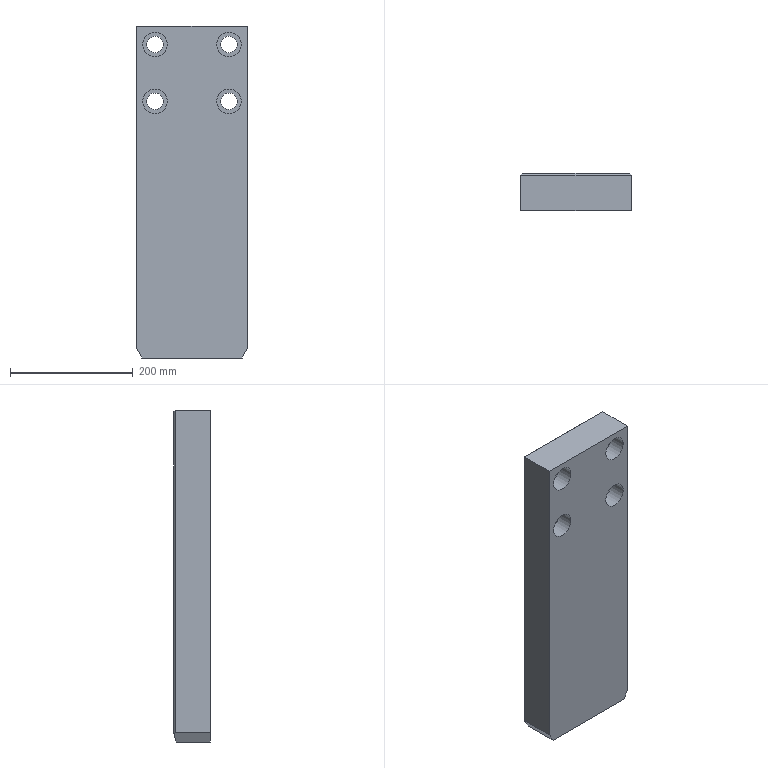Part | NX | features FD 2 | 1 solid | 26 faces | box 180 x 60 x 540 mm | volume 5599611 mm3 | plane 16 | cylinder 9 | cone 1 | commonest cylinder face diameters 27 x4 40 x4 10.2 x1
STEP:
#1=CARTESIAN_POINT('',(2475.,-645.5,147.5));
#2=VERTEX_POINT('',#1);
#3=CARTESIAN_POINT('',(2475.,-645.5,134.));
#4=DIRECTION('',(0.,-1.,0.));
#5=DIRECTION('',(0.,0.,1.));
#6=AXIS2_PLACEMENT_3D('',#3,#4,#5);
#7=CIRCLE('',#6,13.5);
#8=EDGE_CURVE('',#2,#2,#7,.T.);
#9=ORIENTED_EDGE('',*,*,#8,.F.);
#10=EDGE_LOOP('',(#9));
#11=FACE_BOUND('',#10,.T.);
#12=CARTESIAN_POINT('',(2475.,-645.5,154.));
#13=VERTEX_POINT('',#12);
#14=CARTESIAN_POINT('',(2475.,-645.5,134.));
#15=DIRECTION('',(0.,1.,0.));
#16=DIRECTION('',(0.,0.,1.));
#17=AXIS2_PLACEMENT_3D('',#14,#15,#16);
#18=CIRCLE('',#17,20.);
#19=EDGE_CURVE('',#13,#13,#18,.T.);
#20=ORIENTED_EDGE('',*,*,#19,.F.);
#21=EDGE_LOOP('',(#20));
#22=FACE_BOUND('',#21,.T.);
#23=CARTESIAN_POINT('',(2475.,-645.5,134.));
#24=DIRECTION('',(0.,1.,0.));
#25=DIRECTION('',(0.,0.,-1.));
#26=AXIS2_PLACEMENT_3D('',#23,#24,#25);
#27=PLANE('',#26);
#28=ADVANCED_FACE('',(#11,#22),#27,.F.);
#29=CARTESIAN_POINT('',(2475.,-672.5,154.));
#30=VERTEX_POINT('',#29);
#31=CARTESIAN_POINT('',(2475.,-672.5,134.));
#32=DIRECTION('',(0.,1.,0.));
#33=DIRECTION('',(0.,0.,1.));
#34=AXIS2_PLACEMENT_3D('',#31,#32,#33);
#35=CIRCLE('',#34,20.);
#36=EDGE_CURVE('',#30,#30,#35,.T.);
#37=ORIENTED_EDGE('',*,*,#36,.F.);
#38=EDGE_LOOP('',(#37));
#39=FACE_BOUND('',#38,.T.);
#40=ORIENTED_EDGE('',*,*,#19,.T.);
#41=EDGE_LOOP('',(#40));
#42=FACE_BOUND('',#41,.T.);
#43=CARTESIAN_POINT('',(2475.,-656.5,134.));
#44=DIRECTION('',(0.,1.,0.));
#45=DIRECTION('',(0.,0.,-1.));
#46=AXIS2_PLACEMENT_3D('',#43,#44,#45);
#47=CYLINDRICAL_SURFACE('',#46,20.);
#48=ADVANCED_FACE('',(#39,#42),#47,.F.);
#49=ORIENTED_EDGE('',*,*,#8,.T.);
#50=EDGE_LOOP('',(#49));
#51=FACE_BOUND('',#50,.T.);
#52=CARTESIAN_POINT('',(2475.,-612.5,147.5));
#53=VERTEX_POINT('',#52);
#54=CARTESIAN_POINT('',(2475.,-612.5,134.));
#55=DIRECTION('',(0.,1.,0.));
#56=DIRECTION('',(0.,0.,1.));
#57=AXIS2_PLACEMENT_3D('',#54,#55,#56);
#58=CIRCLE('',#57,13.5);
#59=EDGE_CURVE('',#53,#53,#58,.T.);
#60=ORIENTED_EDGE('',*,*,#59,.T.);
#61=EDGE_LOOP('',(#60));
#62=FACE_BOUND('',#61,.T.);
#63=CARTESIAN_POINT('',(2475.,-640.,134.));
#64=DIRECTION('',(0.,1.,0.));
#65=DIRECTION('',(0.,0.,-1.));
#66=AXIS2_PLACEMENT_3D('',#63,#64,#65);
#67=CYLINDRICAL_SURFACE('',#66,13.5);
#68=ADVANCED_FACE('',(#51,#62),#67,.F.);
#69=CARTESIAN_POINT('',(2415.,-637.4,-251.5));
#70=VERTEX_POINT('',#69);
#71=CARTESIAN_POINT('',(2415.,-642.5,-251.5));
#72=DIRECTION('',(0.,0.,1.));
#73=DIRECTION('',(0.,1.,0.));
#74=AXIS2_PLACEMENT_3D('',#71,#72,#73);
#75=CIRCLE('',#74,5.1);
#76=EDGE_CURVE('',#70,#70,#75,.T.);
#77=ORIENTED_EDGE('',*,*,#76,.F.);
#78=EDGE_LOOP('',(#77));
#79=FACE_BOUND('',#78,.T.);
#80=CARTESIAN_POINT('',(2415.,-642.5,-248.556));
#81=VERTEX_POINT('',#80);
#82=VERTEX_LOOP('',#81);
#83=FACE_BOUND('',#82,.T.);
#84=CARTESIAN_POINT('',(2415.,-642.5,-250.028));
#85=DIRECTION('',(0.,0.,-1.));
#86=DIRECTION('',(0.,1.,0.));
#87=AXIS2_PLACEMENT_3D('',#84,#85,#86);
#88=CONICAL_SURFACE('',#87,2.55,1.047);
#89=ADVANCED_FACE('',(#79,#83),#88,.F.);
#90=CARTESIAN_POINT('',(2420.1,-642.5,-283.5));
#91=VERTEX_POINT('',#90);
#92=CARTESIAN_POINT('',(2415.,-642.5,-283.5));
#93=DIRECTION('',(0.,0.,1.));
#94=DIRECTION('',(1.,0.,0.));
#95=AXIS2_PLACEMENT_3D('',#92,#93,#94);
#96=CIRCLE('',#95,5.1);
#97=EDGE_CURVE('',#91,#91,#96,.T.);
#98=ORIENTED_EDGE('',*,*,#97,.F.);
#99=EDGE_LOOP('',(#98));
#100=FACE_BOUND('',#99,.T.);
#101=ORIENTED_EDGE('',*,*,#76,.T.);
#102=EDGE_LOOP('',(#101));
#103=FACE_BOUND('',#102,.T.);
#104=CARTESIAN_POINT('',(2415.,-642.5,-252.25));
#105=DIRECTION('',(0.,0.,1.));
#106=DIRECTION('',(0.,1.,0.));
#107=AXIS2_PLACEMENT_3D('',#104,#105,#106);
#108=CYLINDRICAL_SURFACE('',#107,5.1);
#109=ADVANCED_FACE('',(#100,#103),#108,.F.);
#110=ORIENTED_EDGE('',*,*,#97,.T.);
#111=EDGE_LOOP('',(#110));
#112=FACE_BOUND('',#111,.T.);
#113=CARTESIAN_POINT('',(2333.66,-616.519,-283.5));
#114=VERTEX_POINT('',#113);
#115=CARTESIAN_POINT('',(2496.34,-616.519,-283.5));
#116=VERTEX_POINT('',#115);
#117=CARTESIAN_POINT('',(2415.,-616.519,-283.5));
#118=DIRECTION('',(1.,0.,0.));
#119=VECTOR('',#118,1000.);
#120=LINE('',#117,#119);
#121=EDGE_CURVE('',#114,#116,#120,.T.);
#122=ORIENTED_EDGE('',*,*,#121,.T.);
#123=CARTESIAN_POINT('',(2496.34,-672.5,-283.5));
#124=VERTEX_POINT('',#123);
#125=CARTESIAN_POINT('',(2496.34,-640.,-283.5));
#126=DIRECTION('',(0.,-1.,0.));
#127=VECTOR('',#126,1000.);
#128=LINE('',#125,#127);
#129=EDGE_CURVE('',#116,#124,#128,.T.);
#130=ORIENTED_EDGE('',*,*,#129,.T.);
#131=CARTESIAN_POINT('',(2333.66,-672.5,-283.5));
#132=VERTEX_POINT('',#131);
#133=CARTESIAN_POINT('',(2415.,-672.5,-283.5));
#134=DIRECTION('',(1.,0.,0.));
#135=VECTOR('',#134,1000.);
#136=LINE('',#133,#135);
#137=EDGE_CURVE('',#132,#124,#136,.T.);
#138=ORIENTED_EDGE('',*,*,#137,.F.);
#139=CARTESIAN_POINT('',(2333.66,-640.,-283.5));
#140=DIRECTION('',(0.,1.,0.));
#141=VECTOR('',#140,1000.);
#142=LINE('',#139,#141);
#143=EDGE_CURVE('',#132,#114,#142,.T.);
#144=ORIENTED_EDGE('',*,*,#143,.T.);
#145=EDGE_LOOP('',(#122,#130,#138,#144));
#146=FACE_BOUND('',#145,.T.);
#147=CARTESIAN_POINT('',(2415.,-640.,-283.5));
#148=DIRECTION('',(0.,0.,1.));
#149=DIRECTION('',(0.,1.,0.));
#150=AXIS2_PLACEMENT_3D('',#147,#148,#149);
#151=PLANE('',#150);
#152=ADVANCED_FACE('',(#112,#146),#151,.F.);
#153=CARTESIAN_POINT('',(2502.951,-613.451,-272.049));
#154=VERTEX_POINT('',#153);
#155=CARTESIAN_POINT('',(2502.,-612.5,-268.5));
#156=VERTEX_POINT('',#155);
#157=CARTESIAN_POINT('',(2503.167,-613.667,-272.854));
#158=DIRECTION('',(-0.2506,0.2506,0.9351));
#159=VECTOR('',#158,1000.);
#160=LINE('',#157,#159);
#161=EDGE_CURVE('',#154,#156,#160,.T.);
#162=ORIENTED_EDGE('',*,*,#161,.T.);
#163=CARTESIAN_POINT('',(2502.,-612.5,253.5));
#164=VERTEX_POINT('',#163);
#165=CARTESIAN_POINT('',(2502.,-612.5,1.5));
#166=DIRECTION('',(0.,0.,1.));
#167=VECTOR('',#166,1000.);
#168=LINE('',#165,#167);
#169=EDGE_CURVE('',#156,#164,#168,.T.);
#170=ORIENTED_EDGE('',*,*,#169,.T.);
#171=CARTESIAN_POINT('',(2505.,-615.5,256.5));
#172=VERTEX_POINT('',#171);
#173=CARTESIAN_POINT('',(2443.167,-553.667,194.667));
#174=DIRECTION('',(-0.5774,0.5774,-0.5774));
#175=VECTOR('',#174,1000.);
#176=LINE('',#173,#175);
#177=EDGE_CURVE('',#172,#164,#176,.T.);
#178=ORIENTED_EDGE('',*,*,#177,.F.);
#179=CARTESIAN_POINT('',(2505.,-615.5,-268.5));
#180=VERTEX_POINT('',#179);
#181=CARTESIAN_POINT('',(2505.,-615.5,1.5));
#182=DIRECTION('',(0.,0.,-1.));
#183=VECTOR('',#182,1000.);
#184=LINE('',#181,#183);
#185=EDGE_CURVE('',#172,#180,#184,.T.);
#186=ORIENTED_EDGE('',*,*,#185,.T.);
#187=CARTESIAN_POINT('',(2495.683,-606.183,-284.637));
#188=DIRECTION('',(-0.4472,0.4472,-0.7746));
#189=VECTOR('',#188,1000.);
#190=LINE('',#187,#189);
#191=EDGE_CURVE('',#180,#154,#190,.T.);
#192=ORIENTED_EDGE('',*,*,#191,.T.);
#193=EDGE_LOOP('',(#162,#170,#178,#186,#192));
#194=FACE_BOUND('',#193,.T.);
#195=CARTESIAN_POINT('',(2503.5,-614.,1.5));
#196=DIRECTION('',(0.7071,0.7071,0.));
#197=DIRECTION('',(0.,0.,-1.));
#198=AXIS2_PLACEMENT_3D('',#195,#196,#197);
#199=PLANE('',#198);
#200=ADVANCED_FACE('',(#194),#199,.T.);
#201=ORIENTED_EDGE('',*,*,#177,.T.);
#202=CARTESIAN_POINT('',(2328.,-612.5,253.5));
#203=VERTEX_POINT('',#202);
#204=CARTESIAN_POINT('',(2415.,-612.5,253.5));
#205=DIRECTION('',(-1.,0.,0.));
#206=VECTOR('',#205,1000.);
#207=LINE('',#204,#206);
#208=EDGE_CURVE('',#164,#203,#207,.T.);
#209=ORIENTED_EDGE('',*,*,#208,.T.);
#210=CARTESIAN_POINT('',(2325.,-615.5,256.5));
#211=VERTEX_POINT('',#210);
#212=CARTESIAN_POINT('',(2386.833,-553.667,194.667));
#213=DIRECTION('',(-0.5774,-0.5774,0.5774));
#214=VECTOR('',#213,1000.);
#215=LINE('',#212,#214);
#216=EDGE_CURVE('',#203,#211,#215,.T.);
#217=ORIENTED_EDGE('',*,*,#216,.T.);
#218=CARTESIAN_POINT('',(2415.,-615.5,256.5));
#219=DIRECTION('',(1.,0.,0.));
#220=VECTOR('',#219,1000.);
#221=LINE('',#218,#220);
#222=EDGE_CURVE('',#211,#172,#221,.T.);
#223=ORIENTED_EDGE('',*,*,#222,.T.);
#224=EDGE_LOOP('',(#201,#209,#217,#223));
#225=FACE_BOUND('',#224,.T.);
#226=CARTESIAN_POINT('',(2415.,-614.,255.));
#227=DIRECTION('',(0.,0.7071,0.7071));
#228=DIRECTION('',(0.,0.7071,-0.7071));
#229=AXIS2_PLACEMENT_3D('',#226,#227,#228);
#230=PLANE('',#229);
#231=ADVANCED_FACE('',(#225),#230,.T.);
#232=CARTESIAN_POINT('',(2328.,-612.5,-268.5));
#233=VERTEX_POINT('',#232);
#234=CARTESIAN_POINT('',(2327.049,-613.451,-272.049));
#235=VERTEX_POINT('',#234);
#236=CARTESIAN_POINT('',(2326.833,-613.667,-272.854));
#237=DIRECTION('',(-0.2506,-0.2506,-0.9351));
#238=VECTOR('',#237,1000.);
#239=LINE('',#236,#238);
#240=EDGE_CURVE('',#233,#235,#239,.T.);
#241=ORIENTED_EDGE('',*,*,#240,.T.);
#242=CARTESIAN_POINT('',(2325.,-615.5,-268.5));
#243=VERTEX_POINT('',#242);
#244=CARTESIAN_POINT('',(2334.317,-606.183,-284.637));
#245=DIRECTION('',(-0.4472,-0.4472,0.7746));
#246=VECTOR('',#245,1000.);
#247=LINE('',#244,#246);
#248=EDGE_CURVE('',#235,#243,#247,.T.);
#249=ORIENTED_EDGE('',*,*,#248,.T.);
#250=CARTESIAN_POINT('',(2325.,-615.5,1.5));
#251=DIRECTION('',(0.,0.,1.));
#252=VECTOR('',#251,1000.);
#253=LINE('',#250,#252);
#254=EDGE_CURVE('',#243,#211,#253,.T.);
#255=ORIENTED_EDGE('',*,*,#254,.T.);
#256=ORIENTED_EDGE('',*,*,#216,.F.);
#257=CARTESIAN_POINT('',(2328.,-612.5,1.5));
#258=DIRECTION('',(0.,0.,-1.));
#259=VECTOR('',#258,1000.);
#260=LINE('',#257,#259);
#261=EDGE_CURVE('',#203,#233,#260,.T.);
#262=ORIENTED_EDGE('',*,*,#261,.T.);
#263=EDGE_LOOP('',(#241,#249,#255,#256,#262));
#264=FACE_BOUND('',#263,.T.);
#265=CARTESIAN_POINT('',(2326.5,-614.,1.5));
#266=DIRECTION('',(-0.7071,0.7071,0.));
#267=DIRECTION('',(0.,0.,-1.));
#268=AXIS2_PLACEMENT_3D('',#265,#266,#267);
#269=PLANE('',#268);
#270=ADVANCED_FACE('',(#264),#269,.T.);
#271=ORIENTED_EDGE('',*,*,#161,.F.);
#272=CARTESIAN_POINT('',(2365.709,-677.145,-509.758));
#273=DIRECTION('',(0.4871,0.226,0.8436));
#274=VECTOR('',#273,1000.);
#275=LINE('',#272,#274);
#276=EDGE_CURVE('',#116,#154,#275,.T.);
#277=ORIENTED_EDGE('',*,*,#276,.F.);
#278=ORIENTED_EDGE('',*,*,#121,.F.);
#279=CARTESIAN_POINT('',(2464.291,-677.145,-509.758));
#280=DIRECTION('',(0.4871,-0.226,-0.8436));
#281=VECTOR('',#280,1000.);
#282=LINE('',#279,#281);
#283=EDGE_CURVE('',#235,#114,#282,.T.);
#284=ORIENTED_EDGE('',*,*,#283,.F.);
#285=ORIENTED_EDGE('',*,*,#240,.F.);
#286=CARTESIAN_POINT('',(2415.,-612.5,-268.5));
#287=DIRECTION('',(-1.,0.,0.));
#288=VECTOR('',#287,1000.);
#289=LINE('',#286,#288);
#290=EDGE_CURVE('',#156,#233,#289,.T.);
#291=ORIENTED_EDGE('',*,*,#290,.F.);
#292=EDGE_LOOP('',(#271,#277,#278,#284,#285,#291));
#293=FACE_BOUND('',#292,.T.);
#294=CARTESIAN_POINT('',(2415.,-685.616,-541.374));
#295=DIRECTION('',(0.,0.9659,-0.2588));
#296=DIRECTION('',(0.,-0.2588,-0.9659));
#297=AXIS2_PLACEMENT_3D('',#294,#295,#296);
#298=PLANE('',#297);
#299=ADVANCED_FACE('',(#293),#298,.T.);
#300=CARTESIAN_POINT('',(2355.,-645.5,240.));
#301=VERTEX_POINT('',#300);
#302=CARTESIAN_POINT('',(2355.,-645.5,226.5));
#303=DIRECTION('',(0.,-1.,0.));
#304=DIRECTION('',(0.,0.,1.));
#305=AXIS2_PLACEMENT_3D('',#302,#303,#304);
#306=CIRCLE('',#305,13.5);
#307=EDGE_CURVE('',#301,#301,#306,.T.);
#308=ORIENTED_EDGE('',*,*,#307,.T.);
#309=EDGE_LOOP('',(#308));
#310=FACE_BOUND('',#309,.T.);
#311=CARTESIAN_POINT('',(2355.,-612.5,240.));
#312=VERTEX_POINT('',#311);
#313=CARTESIAN_POINT('',(2355.,-612.5,226.5));
#314=DIRECTION('',(0.,-1.,0.));
#315=DIRECTION('',(0.,0.,1.));
#316=AXIS2_PLACEMENT_3D('',#313,#314,#315);
#317=CIRCLE('',#316,13.5);
#318=EDGE_CURVE('',#312,#312,#317,.T.);
#319=ORIENTED_EDGE('',*,*,#318,.F.);
#320=EDGE_LOOP('',(#319));
#321=FACE_BOUND('',#320,.T.);
#322=CARTESIAN_POINT('',(2355.,-640.,226.5));
#323=DIRECTION('',(0.,1.,0.));
#324=DIRECTION('',(0.,0.,-1.));
#325=AXIS2_PLACEMENT_3D('',#322,#323,#324);
#326=CYLINDRICAL_SURFACE('',#325,13.5);
#327=ADVANCED_FACE('',(#310,#321),#326,.F.);
#328=CARTESIAN_POINT('',(2475.,-645.5,240.));
#329=VERTEX_POINT('',#328);
#330=CARTESIAN_POINT('',(2475.,-645.5,226.5));
#331=DIRECTION('',(0.,-1.,0.));
#332=DIRECTION('',(0.,0.,1.));
#333=AXIS2_PLACEMENT_3D('',#330,#331,#332);
#334=CIRCLE('',#333,13.5);
#335=EDGE_CURVE('',#329,#329,#334,.T.);
#336=ORIENTED_EDGE('',*,*,#335,.T.);
#337=EDGE_LOOP('',(#336));
#338=FACE_BOUND('',#337,.T.);
#339=CARTESIAN_POINT('',(2475.,-612.5,240.));
#340=VERTEX_POINT('',#339);
#341=CARTESIAN_POINT('',(2475.,-612.5,226.5));
#342=DIRECTION('',(0.,-1.,0.));
#343=DIRECTION('',(0.,0.,1.));
#344=AXIS2_PLACEMENT_3D('',#341,#342,#343);
#345=CIRCLE('',#344,13.5);
#346=EDGE_CURVE('',#340,#340,#345,.T.);
#347=ORIENTED_EDGE('',*,*,#346,.F.);
#348=EDGE_LOOP('',(#347));
#349=FACE_BOUND('',#348,.T.);
#350=CARTESIAN_POINT('',(2475.,-640.,226.5));
#351=DIRECTION('',(0.,1.,0.));
#352=DIRECTION('',(0.,0.,-1.));
#353=AXIS2_PLACEMENT_3D('',#350,#351,#352);
#354=CYLINDRICAL_SURFACE('',#353,13.5);
#355=ADVANCED_FACE('',(#338,#349),#354,.F.);
#356=CARTESIAN_POINT('',(2355.,-612.5,147.5));
#357=VERTEX_POINT('',#356);
#358=CARTESIAN_POINT('',(2355.,-612.5,134.));
#359=DIRECTION('',(0.,1.,0.));
#360=DIRECTION('',(0.,0.,1.));
#361=AXIS2_PLACEMENT_3D('',#358,#359,#360);
#362=CIRCLE('',#361,13.5);
#363=EDGE_CURVE('',#357,#357,#362,.T.);
#364=ORIENTED_EDGE('',*,*,#363,.F.);
#365=EDGE_LOOP('',(#364));
#366=FACE_BOUND('',#365,.T.);
#367=ORIENTED_EDGE('',*,*,#59,.F.);
#368=EDGE_LOOP('',(#367));
#369=FACE_BOUND('',#368,.T.);
#370=ORIENTED_EDGE('',*,*,#346,.T.);
#371=EDGE_LOOP('',(#370));
#372=FACE_BOUND('',#371,.T.);
#373=ORIENTED_EDGE('',*,*,#318,.T.);
#374=EDGE_LOOP('',(#373));
#375=FACE_BOUND('',#374,.T.);
#376=ORIENTED_EDGE('',*,*,#290,.T.);
#377=ORIENTED_EDGE('',*,*,#261,.F.);
#378=ORIENTED_EDGE('',*,*,#208,.F.);
#379=ORIENTED_EDGE('',*,*,#169,.F.);
#380=EDGE_LOOP('',(#376,#377,#378,#379));
#381=FACE_BOUND('',#380,.T.);
#382=CARTESIAN_POINT('',(2415.,-612.5,1.5));
#383=DIRECTION('',(0.,1.,0.));
#384=DIRECTION('',(0.,0.,-1.));
#385=AXIS2_PLACEMENT_3D('',#382,#383,#384);
#386=PLANE('',#385);
#387=ADVANCED_FACE('',(#366,#369,#372,#375,#381),#386,.T.);
#388=ORIENTED_EDGE('',*,*,#307,.F.);
#389=EDGE_LOOP('',(#388));
#390=FACE_BOUND('',#389,.T.);
#391=CARTESIAN_POINT('',(2355.,-645.5,246.5));
#392=VERTEX_POINT('',#391);
#393=CARTESIAN_POINT('',(2355.,-645.5,226.5));
#394=DIRECTION('',(0.,1.,0.));
#395=DIRECTION('',(0.,0.,1.));
#396=AXIS2_PLACEMENT_3D('',#393,#394,#395);
#397=CIRCLE('',#396,20.);
#398=EDGE_CURVE('',#392,#392,#397,.T.);
#399=ORIENTED_EDGE('',*,*,#398,.F.);
#400=EDGE_LOOP('',(#399));
#401=FACE_BOUND('',#400,.T.);
#402=CARTESIAN_POINT('',(2355.,-645.5,226.5));
#403=DIRECTION('',(0.,1.,0.));
#404=DIRECTION('',(0.,0.,-1.));
#405=AXIS2_PLACEMENT_3D('',#402,#403,#404);
#406=PLANE('',#405);
#407=ADVANCED_FACE('',(#390,#401),#406,.F.);
#408=ORIENTED_EDGE('',*,*,#335,.F.);
#409=EDGE_LOOP('',(#408));
#410=FACE_BOUND('',#409,.T.);
#411=CARTESIAN_POINT('',(2475.,-645.5,246.5));
#412=VERTEX_POINT('',#411);
#413=CARTESIAN_POINT('',(2475.,-645.5,226.5));
#414=DIRECTION('',(0.,1.,0.));
#415=DIRECTION('',(0.,0.,1.));
#416=AXIS2_PLACEMENT_3D('',#413,#414,#415);
#417=CIRCLE('',#416,20.);
#418=EDGE_CURVE('',#412,#412,#417,.T.);
#419=ORIENTED_EDGE('',*,*,#418,.F.);
#420=EDGE_LOOP('',(#419));
#421=FACE_BOUND('',#420,.T.);
#422=CARTESIAN_POINT('',(2475.,-645.5,226.5));
#423=DIRECTION('',(0.,1.,0.));
#424=DIRECTION('',(0.,0.,-1.));
#425=AXIS2_PLACEMENT_3D('',#422,#423,#424);
#426=PLANE('',#425);
#427=ADVANCED_FACE('',(#410,#421),#426,.F.);
#428=ORIENTED_EDGE('',*,*,#283,.T.);
#429=ORIENTED_EDGE('',*,*,#143,.F.);
#430=CARTESIAN_POINT('',(2325.,-672.5,-268.5));
#431=VERTEX_POINT('',#430);
#432=CARTESIAN_POINT('',(2466.25,-672.5,-513.152));
#433=DIRECTION('',(0.5,0.,-0.866));
#434=VECTOR('',#433,1000.);
#435=LINE('',#432,#434);
#436=EDGE_CURVE('',#431,#132,#435,.T.);
#437=ORIENTED_EDGE('',*,*,#436,.F.);
#438=CARTESIAN_POINT('',(2325.,-640.,-268.5));
#439=DIRECTION('',(0.,-1.,0.));
#440=VECTOR('',#439,1000.);
#441=LINE('',#438,#440);
#442=EDGE_CURVE('',#243,#431,#441,.T.);
#443=ORIENTED_EDGE('',*,*,#442,.F.);
#444=ORIENTED_EDGE('',*,*,#248,.F.);
#445=EDGE_LOOP('',(#428,#429,#437,#443,#444));
#446=FACE_BOUND('',#445,.T.);
#447=CARTESIAN_POINT('',(2466.25,-640.,-513.152));
#448=DIRECTION('',(-0.866,0.,-0.5));
#449=DIRECTION('',(0.,1.,0.));
#450=AXIS2_PLACEMENT_3D('',#447,#448,#449);
#451=PLANE('',#450);
#452=ADVANCED_FACE('',(#446),#451,.T.);
#453=ORIENTED_EDGE('',*,*,#442,.T.);
#454=CARTESIAN_POINT('',(2325.,-672.5,256.5));
#455=VERTEX_POINT('',#454);
#456=CARTESIAN_POINT('',(2325.,-672.5,1.5));
#457=DIRECTION('',(0.,0.,-1.));
#458=VECTOR('',#457,1000.);
#459=LINE('',#456,#458);
#460=EDGE_CURVE('',#455,#431,#459,.T.);
#461=ORIENTED_EDGE('',*,*,#460,.F.);
#462=CARTESIAN_POINT('',(2325.,-640.,256.5));
#463=DIRECTION('',(0.,-1.,0.));
#464=VECTOR('',#463,1000.);
#465=LINE('',#462,#464);
#466=EDGE_CURVE('',#211,#455,#465,.T.);
#467=ORIENTED_EDGE('',*,*,#466,.F.);
#468=ORIENTED_EDGE('',*,*,#254,.F.);
#469=EDGE_LOOP('',(#453,#461,#467,#468));
#470=FACE_BOUND('',#469,.T.);
#471=CARTESIAN_POINT('',(2325.,-640.,1.5));
#472=DIRECTION('',(1.,0.,0.));
#473=DIRECTION('',(0.,-1.,0.));
#474=AXIS2_PLACEMENT_3D('',#471,#472,#473);
#475=PLANE('',#474);
#476=ADVANCED_FACE('',(#470),#475,.F.);
#477=ORIENTED_EDGE('',*,*,#466,.T.);
#478=CARTESIAN_POINT('',(2505.,-672.5,256.5));
#479=VERTEX_POINT('',#478);
#480=CARTESIAN_POINT('',(2415.,-672.5,256.5));
#481=DIRECTION('',(-1.,0.,0.));
#482=VECTOR('',#481,1000.);
#483=LINE('',#480,#482);
#484=EDGE_CURVE('',#479,#455,#483,.T.);
#485=ORIENTED_EDGE('',*,*,#484,.F.);
#486=CARTESIAN_POINT('',(2505.,-640.,256.5));
#487=DIRECTION('',(0.,-1.,0.));
#488=VECTOR('',#487,1000.);
#489=LINE('',#486,#488);
#490=EDGE_CURVE('',#172,#479,#489,.T.);
#491=ORIENTED_EDGE('',*,*,#490,.F.);
#492=ORIENTED_EDGE('',*,*,#222,.F.);
#493=EDGE_LOOP('',(#477,#485,#491,#492));
#494=FACE_BOUND('',#493,.T.);
#495=CARTESIAN_POINT('',(2415.,-640.,256.5));
#496=DIRECTION('',(0.,0.,-1.));
#497=DIRECTION('',(0.,-1.,0.));
#498=AXIS2_PLACEMENT_3D('',#495,#496,#497);
#499=PLANE('',#498);
#500=ADVANCED_FACE('',(#494),#499,.F.);
#501=CARTESIAN_POINT('',(2505.,-672.5,-268.5));
#502=VERTEX_POINT('',#501);
#503=CARTESIAN_POINT('',(2505.,-640.,-268.5));
#504=DIRECTION('',(0.,1.,0.));
#505=VECTOR('',#504,1000.);
#506=LINE('',#503,#505);
#507=EDGE_CURVE('',#502,#180,#506,.T.);
#508=ORIENTED_EDGE('',*,*,#507,.T.);
#509=ORIENTED_EDGE('',*,*,#185,.F.);
#510=ORIENTED_EDGE('',*,*,#490,.T.);
#511=CARTESIAN_POINT('',(2505.,-672.5,1.5));
#512=DIRECTION('',(0.,0.,-1.));
#513=VECTOR('',#512,1000.);
#514=LINE('',#511,#513);
#515=EDGE_CURVE('',#479,#502,#514,.T.);
#516=ORIENTED_EDGE('',*,*,#515,.T.);
#517=EDGE_LOOP('',(#508,#509,#510,#516));
#518=FACE_BOUND('',#517,.T.);
#519=CARTESIAN_POINT('',(2505.,-640.,1.5));
#520=DIRECTION('',(-1.,0.,0.));
#521=DIRECTION('',(0.,1.,0.));
#522=AXIS2_PLACEMENT_3D('',#519,#520,#521);
#523=PLANE('',#522);
#524=ADVANCED_FACE('',(#518),#523,.F.);
#525=ORIENTED_EDGE('',*,*,#276,.T.);
#526=ORIENTED_EDGE('',*,*,#191,.F.);
#527=ORIENTED_EDGE('',*,*,#507,.F.);
#528=CARTESIAN_POINT('',(2363.75,-672.5,-513.152));
#529=DIRECTION('',(0.5,0.,0.866));
#530=VECTOR('',#529,1000.);
#531=LINE('',#528,#530);
#532=EDGE_CURVE('',#124,#502,#531,.T.);
#533=ORIENTED_EDGE('',*,*,#532,.F.);
#534=ORIENTED_EDGE('',*,*,#129,.F.);
#535=EDGE_LOOP('',(#525,#526,#527,#533,#534));
#536=FACE_BOUND('',#535,.T.);
#537=CARTESIAN_POINT('',(2363.75,-640.,-513.152));
#538=DIRECTION('',(0.866,0.,-0.5));
#539=DIRECTION('',(0.,-1.,0.));
#540=AXIS2_PLACEMENT_3D('',#537,#538,#539);
#541=PLANE('',#540);
#542=ADVANCED_FACE('',(#536),#541,.T.);
#543=CARTESIAN_POINT('',(2355.,-672.5,246.5));
#544=VERTEX_POINT('',#543);
#545=CARTESIAN_POINT('',(2355.,-672.5,226.5));
#546=DIRECTION('',(0.,1.,0.));
#547=DIRECTION('',(0.,0.,1.));
#548=AXIS2_PLACEMENT_3D('',#545,#546,#547);
#549=CIRCLE('',#548,20.);
#550=EDGE_CURVE('',#544,#544,#549,.T.);
#551=ORIENTED_EDGE('',*,*,#550,.F.);
#552=EDGE_LOOP('',(#551));
#553=FACE_BOUND('',#552,.T.);
#554=ORIENTED_EDGE('',*,*,#398,.T.);
#555=EDGE_LOOP('',(#554));
#556=FACE_BOUND('',#555,.T.);
#557=CARTESIAN_POINT('',(2355.,-656.5,226.5));
#558=DIRECTION('',(0.,1.,0.));
#559=DIRECTION('',(0.,0.,-1.));
#560=AXIS2_PLACEMENT_3D('',#557,#558,#559);
#561=CYLINDRICAL_SURFACE('',#560,20.);
#562=ADVANCED_FACE('',(#553,#556),#561,.F.);
#563=CARTESIAN_POINT('',(2475.,-672.5,246.5));
#564=VERTEX_POINT('',#563);
#565=CARTESIAN_POINT('',(2475.,-672.5,226.5));
#566=DIRECTION('',(0.,1.,0.));
#567=DIRECTION('',(0.,0.,1.));
#568=AXIS2_PLACEMENT_3D('',#565,#566,#567);
#569=CIRCLE('',#568,20.);
#570=EDGE_CURVE('',#564,#564,#569,.T.);
#571=ORIENTED_EDGE('',*,*,#570,.F.);
#572=EDGE_LOOP('',(#571));
#573=FACE_BOUND('',#572,.T.);
#574=ORIENTED_EDGE('',*,*,#418,.T.);
#575=EDGE_LOOP('',(#574));
#576=FACE_BOUND('',#575,.T.);
#577=CARTESIAN_POINT('',(2475.,-656.5,226.5));
#578=DIRECTION('',(0.,1.,0.));
#579=DIRECTION('',(0.,0.,-1.));
#580=AXIS2_PLACEMENT_3D('',#577,#578,#579);
#581=CYLINDRICAL_SURFACE('',#580,20.);
#582=ADVANCED_FACE('',(#573,#576),#581,.F.);
#583=CARTESIAN_POINT('',(2355.,-672.5,154.));
#584=VERTEX_POINT('',#583);
#585=CARTESIAN_POINT('',(2355.,-672.5,134.));
#586=DIRECTION('',(0.,1.,0.));
#587=DIRECTION('',(0.,0.,1.));
#588=AXIS2_PLACEMENT_3D('',#585,#586,#587);
#589=CIRCLE('',#588,20.);
#590=EDGE_CURVE('',#584,#584,#589,.T.);
#591=ORIENTED_EDGE('',*,*,#590,.T.);
#592=EDGE_LOOP('',(#591));
#593=FACE_BOUND('',#592,.T.);
#594=ORIENTED_EDGE('',*,*,#36,.T.);
#595=EDGE_LOOP('',(#594));
#596=FACE_BOUND('',#595,.T.);
#597=ORIENTED_EDGE('',*,*,#570,.T.);
#598=EDGE_LOOP('',(#597));
#599=FACE_BOUND('',#598,.T.);
#600=ORIENTED_EDGE('',*,*,#550,.T.);
#601=EDGE_LOOP('',(#600));
#602=FACE_BOUND('',#601,.T.);
#603=ORIENTED_EDGE('',*,*,#532,.T.);
#604=ORIENTED_EDGE('',*,*,#515,.F.);
#605=ORIENTED_EDGE('',*,*,#484,.T.);
#606=ORIENTED_EDGE('',*,*,#460,.T.);
#607=ORIENTED_EDGE('',*,*,#436,.T.);
#608=ORIENTED_EDGE('',*,*,#137,.T.);
#609=EDGE_LOOP('',(#603,#604,#605,#606,#607,#608));
#610=FACE_BOUND('',#609,.T.);
#611=CARTESIAN_POINT('',(2415.,-672.5,1.5));
#612=DIRECTION('',(0.,1.,0.));
#613=DIRECTION('',(0.,0.,-1.));
#614=AXIS2_PLACEMENT_3D('',#611,#612,#613);
#615=PLANE('',#614);
#616=ADVANCED_FACE('',(#593,#596,#599,#602,#610),#615,.F.);
#617=CARTESIAN_POINT('',(2355.,-645.5,147.5));
#618=VERTEX_POINT('',#617);
#619=CARTESIAN_POINT('',(2355.,-645.5,134.));
#620=DIRECTION('',(0.,-1.,0.));
#621=DIRECTION('',(0.,0.,1.));
#622=AXIS2_PLACEMENT_3D('',#619,#620,#621);
#623=CIRCLE('',#622,13.5);
#624=EDGE_CURVE('',#618,#618,#623,.T.);
#625=ORIENTED_EDGE('',*,*,#624,.F.);
#626=EDGE_LOOP('',(#625));
#627=FACE_BOUND('',#626,.T.);
#628=CARTESIAN_POINT('',(2355.,-645.5,154.));
#629=VERTEX_POINT('',#628);
#630=CARTESIAN_POINT('',(2355.,-645.5,134.));
#631=DIRECTION('',(0.,1.,0.));
#632=DIRECTION('',(0.,0.,1.));
#633=AXIS2_PLACEMENT_3D('',#630,#631,#632);
#634=CIRCLE('',#633,20.);
#635=EDGE_CURVE('',#629,#629,#634,.T.);
#636=ORIENTED_EDGE('',*,*,#635,.F.);
#637=EDGE_LOOP('',(#636));
#638=FACE_BOUND('',#637,.T.);
#639=CARTESIAN_POINT('',(2355.,-645.5,134.));
#640=DIRECTION('',(0.,1.,0.));
#641=DIRECTION('',(0.,0.,-1.));
#642=AXIS2_PLACEMENT_3D('',#639,#640,#641);
#643=PLANE('',#642);
#644=ADVANCED_FACE('',(#627,#638),#643,.F.);
#645=ORIENTED_EDGE('',*,*,#590,.F.);
#646=EDGE_LOOP('',(#645));
#647=FACE_BOUND('',#646,.T.);
#648=ORIENTED_EDGE('',*,*,#635,.T.);
#649=EDGE_LOOP('',(#648));
#650=FACE_BOUND('',#649,.T.);
#651=CARTESIAN_POINT('',(2355.,-656.5,134.));
#652=DIRECTION('',(0.,1.,0.));
#653=DIRECTION('',(0.,0.,-1.));
#654=AXIS2_PLACEMENT_3D('',#651,#652,#653);
#655=CYLINDRICAL_SURFACE('',#654,20.);
#656=ADVANCED_FACE('',(#647,#650),#655,.F.);
#657=ORIENTED_EDGE('',*,*,#624,.T.);
#658=EDGE_LOOP('',(#657));
#659=FACE_BOUND('',#658,.T.);
#660=ORIENTED_EDGE('',*,*,#363,.T.);
#661=EDGE_LOOP('',(#660));
#662=FACE_BOUND('',#661,.T.);
#663=CARTESIAN_POINT('',(2355.,-640.,134.));
#664=DIRECTION('',(0.,1.,0.));
#665=DIRECTION('',(0.,0.,-1.));
#666=AXIS2_PLACEMENT_3D('',#663,#664,#665);
#667=CYLINDRICAL_SURFACE('',#666,13.5);
#668=ADVANCED_FACE('',(#659,#662),#667,.F.);
#669=CLOSED_SHELL('',(#28,#48,#68,#89,#109,#152,#200,#231,#270,#299,#327,#355,#387,#407,#427,#452,#476,#500,#524,#542,#562,#582,#616,#644,#656,#668));
#670=MANIFOLD_SOLID_BREP('',#669);
#671=(LENGTH_UNIT()NAMED_UNIT(*)SI_UNIT(.MILLI.,.METRE.));
#672=UNCERTAINTY_MEASURE_WITH_UNIT(LENGTH_MEASURE(0.00001),#671,'','');
#673=(NAMED_UNIT(*)PLANE_ANGLE_UNIT()SI_UNIT($,.RADIAN.));
#674=(NAMED_UNIT(*)SI_UNIT($,.STERADIAN.)SOLID_ANGLE_UNIT());
#675=(GEOMETRIC_REPRESENTATION_CONTEXT(3)GLOBAL_UNCERTAINTY_ASSIGNED_CONTEXT((#672))GLOBAL_UNIT_ASSIGNED_CONTEXT((#671,#673,#674))REPRESENTATION_CONTEXT('',''));
#676=ADVANCED_BREP_SHAPE_REPRESENTATION('',(#670),#675);